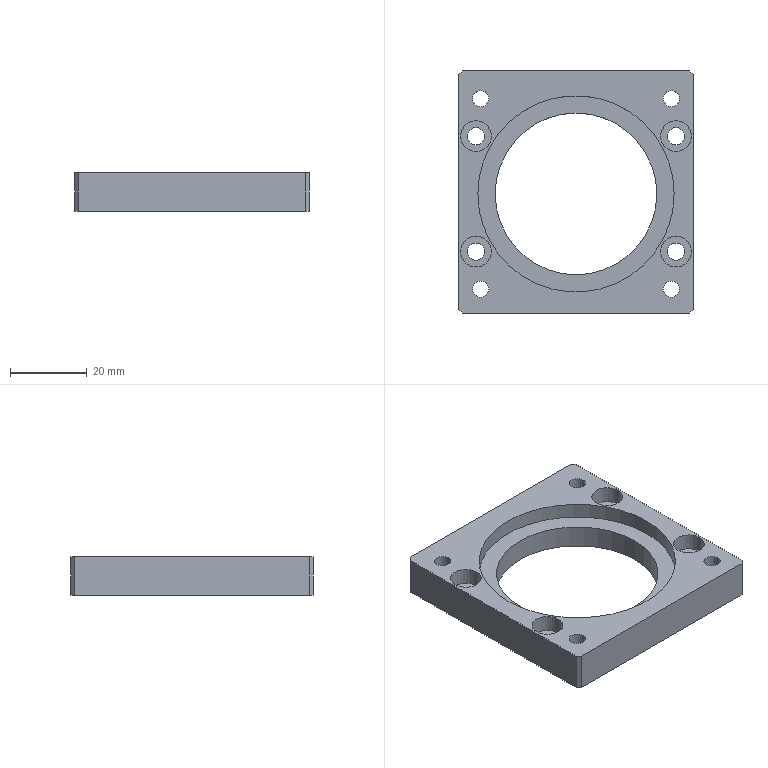Part | STEP file | 1 solid | 43 faces | box 61 x 63 x 10 mm | volume 20131 mm3 | cylinder 28 | plane 15 | commonest cylinder face diameters 4.2 x8 4.5 x8 8 x8 42 x2 51 x2